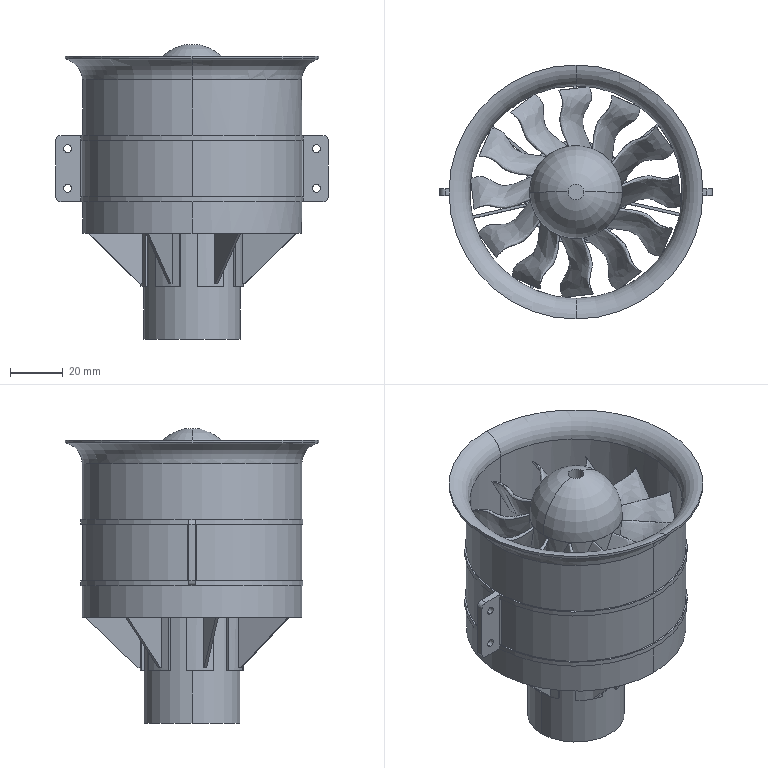Part | SolidWorks | features CompositeCurve 2 | 4 solids | 253 faces | box 103 x 96 x 111.255 mm | volume 142445 mm3 | plane 139 | cylinder 77 | spline 24 | cone 7 | torus 6 | commonest cylinder face diameters 12.5 x12 31 x12 3 x8 83 x7 84.2 x6 1 x4